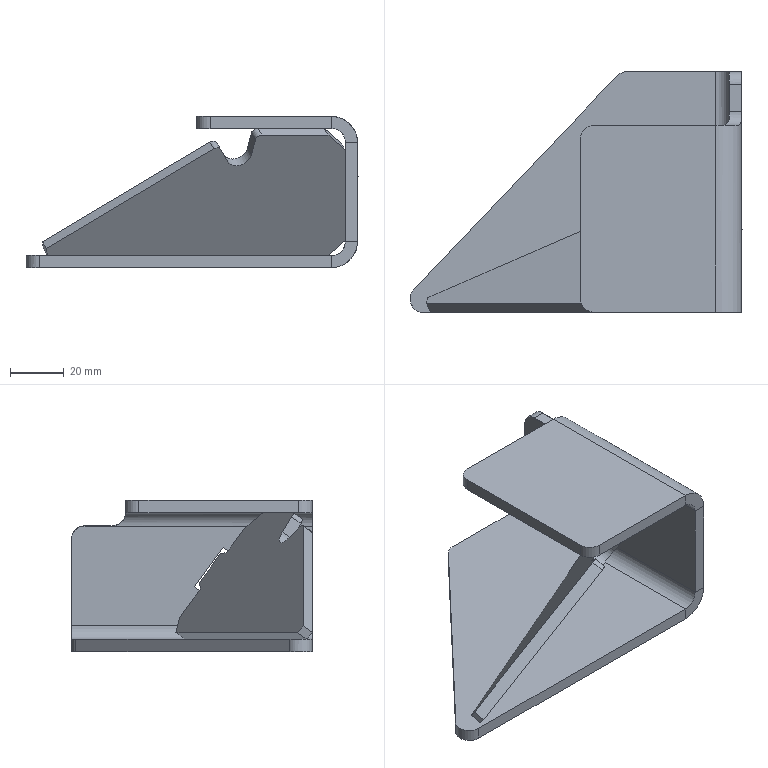Part | SolidWorks | features MBimport 1 | 2 solids | 51 faces | box 123.265 x 89.4 x 56.1 mm | volume 89195 mm3 | plane 38 | cylinder 13 | commonest cylinder face diameters 10 x9 4 x2 19 x2